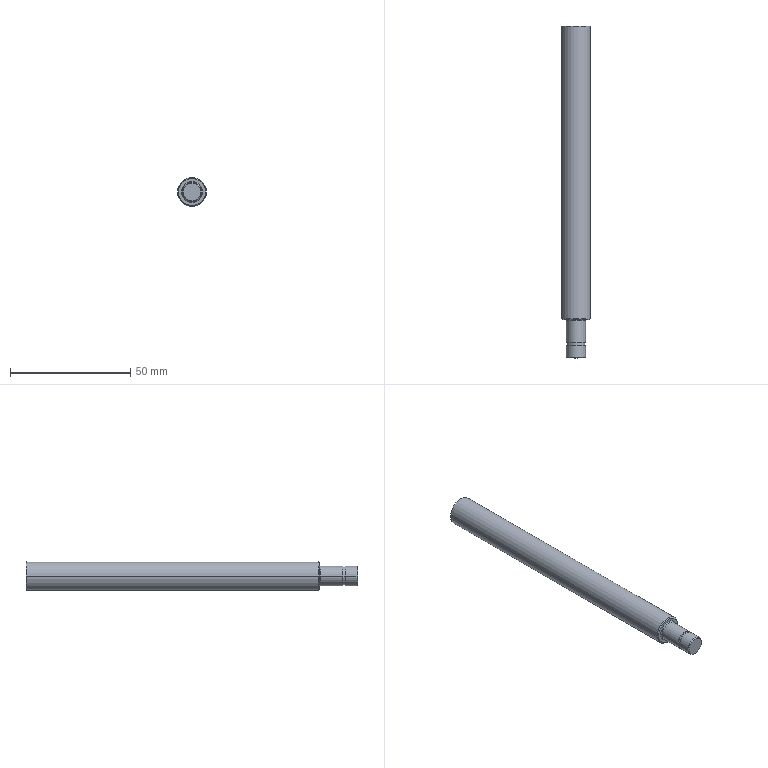Part | NX | features BREP 1 | 1 solid | 19 faces | box 12 x 138 x 12 mm | volume 14591 mm3 | cylinder 8 | plane 5 | cone 4 | torus 2 | commonest cylinder face diameters 8 x4 7.4 x2 12 x2
STEP:
#1=CARTESIAN_POINT('',(-6.,81.4,0.));
#2=VERTEX_POINT('',#1);
#3=CARTESIAN_POINT('',(-6.,203.,0.));
#4=VERTEX_POINT('',#3);
#5=CARTESIAN_POINT('',(-6.,65.,0.));
#6=DIRECTION('',(0.,1.,0.));
#7=VECTOR('',#6,1000.);
#8=LINE('',#5,#7);
#9=EDGE_CURVE('',#2,#4,#8,.T.);
#10=ORIENTED_EDGE('',*,*,#9,.T.);
#11=CARTESIAN_POINT('',(6.,203.,0.));
#12=VERTEX_POINT('',#11);
#13=CARTESIAN_POINT('',(0.,203.,0.));
#14=DIRECTION('',(0.,-1.,0.));
#15=DIRECTION('',(1.,0.,0.));
#16=AXIS2_PLACEMENT_3D('',#13,#14,#15);
#17=CIRCLE('',#16,6.);
#18=EDGE_CURVE('',#4,#12,#17,.T.);
#19=ORIENTED_EDGE('',*,*,#18,.T.);
#20=CARTESIAN_POINT('',(6.,81.4,0.));
#21=VERTEX_POINT('',#20);
#22=CARTESIAN_POINT('',(6.,65.,0.));
#23=DIRECTION('',(0.,-1.,0.));
#24=VECTOR('',#23,1000.);
#25=LINE('',#22,#24);
#26=EDGE_CURVE('',#12,#21,#25,.T.);
#27=ORIENTED_EDGE('',*,*,#26,.T.);
#28=CARTESIAN_POINT('',(0.,81.4,0.));
#29=DIRECTION('',(0.,1.,0.));
#30=DIRECTION('',(-1.,0.,0.));
#31=AXIS2_PLACEMENT_3D('',#28,#29,#30);
#32=CIRCLE('',#31,6.);
#33=EDGE_CURVE('',#21,#2,#32,.T.);
#34=ORIENTED_EDGE('',*,*,#33,.T.);
#35=EDGE_LOOP('',(#10,#19,#27,#34));
#36=FACE_BOUND('',#35,.T.);
#37=CARTESIAN_POINT('',(0.,65.,0.));
#38=DIRECTION('',(0.,-1.,0.));
#39=DIRECTION('',(1.,0.,0.));
#40=AXIS2_PLACEMENT_3D('',#37,#38,#39);
#41=CYLINDRICAL_SURFACE('',#40,6.);
#42=ADVANCED_FACE('',(#36),#41,.T.);
#43=ORIENTED_EDGE('',*,*,#26,.F.);
#44=CARTESIAN_POINT('',(0.,203.,0.));
#45=DIRECTION('',(0.,-1.,0.));
#46=DIRECTION('',(1.,0.,0.));
#47=AXIS2_PLACEMENT_3D('',#44,#45,#46);
#48=CIRCLE('',#47,6.);
#49=EDGE_CURVE('',#12,#4,#48,.T.);
#50=ORIENTED_EDGE('',*,*,#49,.T.);
#51=ORIENTED_EDGE('',*,*,#9,.F.);
#52=CARTESIAN_POINT('',(0.,81.4,0.));
#53=DIRECTION('',(0.,1.,0.));
#54=DIRECTION('',(-1.,0.,0.));
#55=AXIS2_PLACEMENT_3D('',#52,#53,#54);
#56=CIRCLE('',#55,6.);
#57=EDGE_CURVE('',#2,#21,#56,.T.);
#58=ORIENTED_EDGE('',*,*,#57,.T.);
#59=EDGE_LOOP('',(#43,#50,#51,#58));
#60=FACE_BOUND('',#59,.T.);
#61=CARTESIAN_POINT('',(0.,65.,0.));
#62=DIRECTION('',(0.,-1.,0.));
#63=DIRECTION('',(1.,0.,0.));
#64=AXIS2_PLACEMENT_3D('',#61,#62,#63);
#65=CYLINDRICAL_SURFACE('',#64,6.);
#66=ADVANCED_FACE('',(#60),#65,.T.);
#67=CARTESIAN_POINT('',(4.,80.6,0.));
#68=VERTEX_POINT('',#67);
#69=CARTESIAN_POINT('',(-4.,80.6,0.));
#70=VERTEX_POINT('',#69);
#71=CARTESIAN_POINT('',(0.,80.6,0.));
#72=DIRECTION('',(0.,-1.,0.));
#73=DIRECTION('',(-1.,0.,0.));
#74=AXIS2_PLACEMENT_3D('',#71,#72,#73);
#75=CIRCLE('',#74,4.);
#76=EDGE_CURVE('',#68,#70,#75,.T.);
#77=ORIENTED_EDGE('',*,*,#76,.F.);
#78=CARTESIAN_POINT('',(4.4,81.,0.));
#79=VERTEX_POINT('',#78);
#80=CARTESIAN_POINT('',(4.4,80.6,0.));
#81=DIRECTION('',(0.,0.,1.));
#82=DIRECTION('',(-1.,0.,0.));
#83=AXIS2_PLACEMENT_3D('',#80,#81,#82);
#84=CIRCLE('',#83,0.4);
#85=EDGE_CURVE('',#79,#68,#84,.T.);
#86=ORIENTED_EDGE('',*,*,#85,.F.);
#87=CARTESIAN_POINT('',(-4.4,81.,0.));
#88=VERTEX_POINT('',#87);
#89=CARTESIAN_POINT('',(0.,81.,0.));
#90=DIRECTION('',(0.,1.,0.));
#91=DIRECTION('',(-1.,0.,0.));
#92=AXIS2_PLACEMENT_3D('',#89,#90,#91);
#93=CIRCLE('',#92,4.4);
#94=EDGE_CURVE('',#88,#79,#93,.T.);
#95=ORIENTED_EDGE('',*,*,#94,.F.);
#96=CARTESIAN_POINT('',(-4.4,80.6,0.));
#97=DIRECTION('',(0.,0.,1.));
#98=DIRECTION('',(1.,0.,0.));
#99=AXIS2_PLACEMENT_3D('',#96,#97,#98);
#100=CIRCLE('',#99,0.4);
#101=EDGE_CURVE('',#70,#88,#100,.T.);
#102=ORIENTED_EDGE('',*,*,#101,.F.);
#103=EDGE_LOOP('',(#77,#86,#95,#102));
#104=FACE_BOUND('',#103,.T.);
#105=CARTESIAN_POINT('',(0.,80.6,0.));
#106=DIRECTION('',(0.,-1.,0.));
#107=DIRECTION('',(1.,0.,0.));
#108=AXIS2_PLACEMENT_3D('',#105,#106,#107);
#109=TOROIDAL_SURFACE('',#108,4.4,0.4);
#110=ADVANCED_FACE('',(#104),#109,.F.);
#111=CARTESIAN_POINT('',(-5.6,81.,0.));
#112=VERTEX_POINT('',#111);
#113=CARTESIAN_POINT('',(5.6,81.,0.));
#114=VERTEX_POINT('',#113);
#115=CARTESIAN_POINT('',(0.,81.,0.));
#116=DIRECTION('',(0.,-1.,0.));
#117=DIRECTION('',(-1.,0.,0.));
#118=AXIS2_PLACEMENT_3D('',#115,#116,#117);
#119=CIRCLE('',#118,5.6);
#120=EDGE_CURVE('',#112,#114,#119,.T.);
#121=ORIENTED_EDGE('',*,*,#120,.F.);
#122=CARTESIAN_POINT('',(-5.6,81.,0.));
#123=DIRECTION('',(-0.7071,0.7071,0.));
#124=VECTOR('',#123,1000.);
#125=LINE('',#122,#124);
#126=EDGE_CURVE('',#112,#2,#125,.T.);
#127=ORIENTED_EDGE('',*,*,#126,.T.);
#128=ORIENTED_EDGE('',*,*,#33,.F.);
#129=CARTESIAN_POINT('',(5.6,81.,0.));
#130=DIRECTION('',(-0.7071,-0.7071,0.));
#131=VECTOR('',#130,1000.);
#132=LINE('',#129,#131);
#133=EDGE_CURVE('',#21,#114,#132,.T.);
#134=ORIENTED_EDGE('',*,*,#133,.T.);
#135=EDGE_LOOP('',(#121,#127,#128,#134));
#136=FACE_BOUND('',#135,.T.);
#137=CARTESIAN_POINT('',(0.,81.,0.));
#138=DIRECTION('',(0.,1.,0.));
#139=DIRECTION('',(-1.,0.,0.));
#140=AXIS2_PLACEMENT_3D('',#137,#138,#139);
#141=CONICAL_SURFACE('',#140,5.6,0.7854);
#142=ADVANCED_FACE('',(#136),#141,.T.);
#143=CARTESIAN_POINT('',(-3.6,65.,0.));
#144=VERTEX_POINT('',#143);
#145=CARTESIAN_POINT('',(3.6,65.,0.));
#146=VERTEX_POINT('',#145);
#147=CARTESIAN_POINT('',(0.,65.,0.));
#148=DIRECTION('',(0.,-1.,0.));
#149=DIRECTION('',(-1.,0.,0.));
#150=AXIS2_PLACEMENT_3D('',#147,#148,#149);
#151=CIRCLE('',#150,3.6);
#152=EDGE_CURVE('',#144,#146,#151,.T.);
#153=ORIENTED_EDGE('',*,*,#152,.F.);
#154=CARTESIAN_POINT('',(-4.,65.4,0.));
#155=VERTEX_POINT('',#154);
#156=CARTESIAN_POINT('',(-3.6,65.,0.));
#157=DIRECTION('',(-0.7071,0.7071,0.));
#158=VECTOR('',#157,1000.);
#159=LINE('',#156,#158);
#160=EDGE_CURVE('',#144,#155,#159,.T.);
#161=ORIENTED_EDGE('',*,*,#160,.T.);
#162=CARTESIAN_POINT('',(4.,65.4,0.));
#163=VERTEX_POINT('',#162);
#164=CARTESIAN_POINT('',(0.,65.4,0.));
#165=DIRECTION('',(0.,1.,0.));
#166=DIRECTION('',(-1.,0.,0.));
#167=AXIS2_PLACEMENT_3D('',#164,#165,#166);
#168=CIRCLE('',#167,4.);
#169=EDGE_CURVE('',#163,#155,#168,.T.);
#170=ORIENTED_EDGE('',*,*,#169,.F.);
#171=CARTESIAN_POINT('',(3.6,65.,0.));
#172=DIRECTION('',(-0.7071,-0.7071,0.));
#173=VECTOR('',#172,1000.);
#174=LINE('',#171,#173);
#175=EDGE_CURVE('',#163,#146,#174,.T.);
#176=ORIENTED_EDGE('',*,*,#175,.T.);
#177=EDGE_LOOP('',(#153,#161,#170,#176));
#178=FACE_BOUND('',#177,.T.);
#179=CARTESIAN_POINT('',(0.,65.,0.));
#180=DIRECTION('',(0.,1.,0.));
#181=DIRECTION('',(-1.,0.,0.));
#182=AXIS2_PLACEMENT_3D('',#179,#180,#181);
#183=CONICAL_SURFACE('',#182,3.6,0.7854);
#184=ADVANCED_FACE('',(#178),#183,.T.);
#185=CARTESIAN_POINT('',(-4.,70.3,0.));
#186=VERTEX_POINT('',#185);
#187=CARTESIAN_POINT('',(4.,70.3,0.));
#188=VERTEX_POINT('',#187);
#189=CARTESIAN_POINT('',(0.,70.3,0.));
#190=DIRECTION('',(0.,-1.,0.));
#191=DIRECTION('',(-1.,0.,0.));
#192=AXIS2_PLACEMENT_3D('',#189,#190,#191);
#193=CIRCLE('',#192,4.);
#194=EDGE_CURVE('',#186,#188,#193,.T.);
#195=ORIENTED_EDGE('',*,*,#194,.T.);
#196=CARTESIAN_POINT('',(4.,65.,0.));
#197=DIRECTION('',(0.,1.,0.));
#198=VECTOR('',#197,1000.);
#199=LINE('',#196,#198);
#200=EDGE_CURVE('',#163,#188,#199,.T.);
#201=ORIENTED_EDGE('',*,*,#200,.F.);
#202=ORIENTED_EDGE('',*,*,#169,.T.);
#203=CARTESIAN_POINT('',(-4.,65.,0.));
#204=DIRECTION('',(0.,-1.,0.));
#205=VECTOR('',#204,1000.);
#206=LINE('',#203,#205);
#207=EDGE_CURVE('',#186,#155,#206,.T.);
#208=ORIENTED_EDGE('',*,*,#207,.F.);
#209=EDGE_LOOP('',(#195,#201,#202,#208));
#210=FACE_BOUND('',#209,.T.);
#211=CARTESIAN_POINT('',(0.,65.,0.));
#212=DIRECTION('',(0.,-1.,0.));
#213=DIRECTION('',(1.,0.,0.));
#214=AXIS2_PLACEMENT_3D('',#211,#212,#213);
#215=CYLINDRICAL_SURFACE('',#214,4.);
#216=ADVANCED_FACE('',(#210),#215,.T.);
#217=CARTESIAN_POINT('',(-3.7,71.3,0.));
#218=VERTEX_POINT('',#217);
#219=CARTESIAN_POINT('',(3.7,71.3,0.));
#220=VERTEX_POINT('',#219);
#221=CARTESIAN_POINT('',(0.,71.3,0.));
#222=DIRECTION('',(0.,-1.,0.));
#223=DIRECTION('',(-1.,0.,0.));
#224=AXIS2_PLACEMENT_3D('',#221,#222,#223);
#225=CIRCLE('',#224,3.7);
#226=EDGE_CURVE('',#218,#220,#225,.T.);
#227=ORIENTED_EDGE('',*,*,#226,.T.);
#228=CARTESIAN_POINT('',(3.7,70.3,0.));
#229=VERTEX_POINT('',#228);
#230=CARTESIAN_POINT('',(3.7,65.,0.));
#231=DIRECTION('',(0.,1.,0.));
#232=VECTOR('',#231,1000.);
#233=LINE('',#230,#232);
#234=EDGE_CURVE('',#229,#220,#233,.T.);
#235=ORIENTED_EDGE('',*,*,#234,.F.);
#236=CARTESIAN_POINT('',(-3.7,70.3,0.));
#237=VERTEX_POINT('',#236);
#238=CARTESIAN_POINT('',(0.,70.3,0.));
#239=DIRECTION('',(0.,-1.,0.));
#240=DIRECTION('',(-1.,0.,0.));
#241=AXIS2_PLACEMENT_3D('',#238,#239,#240);
#242=CIRCLE('',#241,3.7);
#243=EDGE_CURVE('',#237,#229,#242,.T.);
#244=ORIENTED_EDGE('',*,*,#243,.F.);
#245=CARTESIAN_POINT('',(-3.7,65.,0.));
#246=DIRECTION('',(0.,-1.,0.));
#247=VECTOR('',#246,1000.);
#248=LINE('',#245,#247);
#249=EDGE_CURVE('',#218,#237,#248,.T.);
#250=ORIENTED_EDGE('',*,*,#249,.F.);
#251=EDGE_LOOP('',(#227,#235,#244,#250));
#252=FACE_BOUND('',#251,.T.);
#253=CARTESIAN_POINT('',(0.,65.,0.));
#254=DIRECTION('',(0.,-1.,0.));
#255=DIRECTION('',(1.,0.,0.));
#256=AXIS2_PLACEMENT_3D('',#253,#254,#255);
#257=CYLINDRICAL_SURFACE('',#256,3.7);
#258=ADVANCED_FACE('',(#252),#257,.T.);
#259=CARTESIAN_POINT('',(0.,80.6,0.));
#260=DIRECTION('',(0.,-1.,0.));
#261=DIRECTION('',(-1.,0.,0.));
#262=AXIS2_PLACEMENT_3D('',#259,#260,#261);
#263=CIRCLE('',#262,4.);
#264=EDGE_CURVE('',#70,#68,#263,.T.);
#265=ORIENTED_EDGE('',*,*,#264,.T.);
#266=CARTESIAN_POINT('',(4.,71.3,0.));
#267=VERTEX_POINT('',#266);
#268=CARTESIAN_POINT('',(4.,65.,0.));
#269=DIRECTION('',(0.,1.,0.));
#270=VECTOR('',#269,1000.);
#271=LINE('',#268,#270);
#272=EDGE_CURVE('',#267,#68,#271,.T.);
#273=ORIENTED_EDGE('',*,*,#272,.F.);
#274=CARTESIAN_POINT('',(-4.,71.3,0.));
#275=VERTEX_POINT('',#274);
#276=CARTESIAN_POINT('',(0.,71.3,0.));
#277=DIRECTION('',(0.,-1.,0.));
#278=DIRECTION('',(-1.,0.,0.));
#279=AXIS2_PLACEMENT_3D('',#276,#277,#278);
#280=CIRCLE('',#279,4.);
#281=EDGE_CURVE('',#275,#267,#280,.T.);
#282=ORIENTED_EDGE('',*,*,#281,.F.);
#283=CARTESIAN_POINT('',(-4.,65.,0.));
#284=DIRECTION('',(0.,-1.,0.));
#285=VECTOR('',#284,1000.);
#286=LINE('',#283,#285);
#287=EDGE_CURVE('',#70,#275,#286,.T.);
#288=ORIENTED_EDGE('',*,*,#287,.F.);
#289=EDGE_LOOP('',(#265,#273,#282,#288));
#290=FACE_BOUND('',#289,.T.);
#291=CARTESIAN_POINT('',(0.,65.,0.));
#292=DIRECTION('',(0.,-1.,0.));
#293=DIRECTION('',(1.,0.,0.));
#294=AXIS2_PLACEMENT_3D('',#291,#292,#293);
#295=CYLINDRICAL_SURFACE('',#294,4.);
#296=ADVANCED_FACE('',(#290),#295,.T.);
#297=ORIENTED_EDGE('',*,*,#272,.T.);
#298=ORIENTED_EDGE('',*,*,#76,.T.);
#299=ORIENTED_EDGE('',*,*,#287,.T.);
#300=CARTESIAN_POINT('',(0.,71.3,0.));
#301=DIRECTION('',(0.,-1.,0.));
#302=DIRECTION('',(-1.,0.,0.));
#303=AXIS2_PLACEMENT_3D('',#300,#301,#302);
#304=CIRCLE('',#303,4.);
#305=EDGE_CURVE('',#267,#275,#304,.T.);
#306=ORIENTED_EDGE('',*,*,#305,.F.);
#307=EDGE_LOOP('',(#297,#298,#299,#306));
#308=FACE_BOUND('',#307,.T.);
#309=CARTESIAN_POINT('',(0.,65.,0.));
#310=DIRECTION('',(0.,-1.,0.));
#311=DIRECTION('',(1.,0.,0.));
#312=AXIS2_PLACEMENT_3D('',#309,#310,#311);
#313=CYLINDRICAL_SURFACE('',#312,4.);
#314=ADVANCED_FACE('',(#308),#313,.T.);
#315=ORIENTED_EDGE('',*,*,#226,.F.);
#316=CARTESIAN_POINT('',(0.,71.3,0.));
#317=DIRECTION('',(0.,-1.,0.));
#318=DIRECTION('',(-1.,0.,0.));
#319=AXIS2_PLACEMENT_3D('',#316,#317,#318);
#320=CIRCLE('',#319,3.7);
#321=EDGE_CURVE('',#220,#218,#320,.T.);
#322=ORIENTED_EDGE('',*,*,#321,.F.);
#323=EDGE_LOOP('',(#315,#322));
#324=FACE_BOUND('',#323,.T.);
#325=ORIENTED_EDGE('',*,*,#281,.T.);
#326=ORIENTED_EDGE('',*,*,#305,.T.);
#327=EDGE_LOOP('',(#325,#326));
#328=FACE_BOUND('',#327,.T.);
#329=CARTESIAN_POINT('',(0.,71.3,0.));
#330=DIRECTION('',(0.,1.,0.));
#331=DIRECTION('',(-1.,0.,0.));
#332=AXIS2_PLACEMENT_3D('',#329,#330,#331);
#333=PLANE('',#332);
#334=ADVANCED_FACE('',(#324,#328),#333,.F.);
#335=ORIENTED_EDGE('',*,*,#234,.T.);
#336=ORIENTED_EDGE('',*,*,#321,.T.);
#337=ORIENTED_EDGE('',*,*,#249,.T.);
#338=CARTESIAN_POINT('',(0.,70.3,0.));
#339=DIRECTION('',(0.,-1.,0.));
#340=DIRECTION('',(-1.,0.,0.));
#341=AXIS2_PLACEMENT_3D('',#338,#339,#340);
#342=CIRCLE('',#341,3.7);
#343=EDGE_CURVE('',#229,#237,#342,.T.);
#344=ORIENTED_EDGE('',*,*,#343,.F.);
#345=EDGE_LOOP('',(#335,#336,#337,#344));
#346=FACE_BOUND('',#345,.T.);
#347=CARTESIAN_POINT('',(0.,65.,0.));
#348=DIRECTION('',(0.,-1.,0.));
#349=DIRECTION('',(1.,0.,0.));
#350=AXIS2_PLACEMENT_3D('',#347,#348,#349);
#351=CYLINDRICAL_SURFACE('',#350,3.7);
#352=ADVANCED_FACE('',(#346),#351,.T.);
#353=ORIENTED_EDGE('',*,*,#243,.T.);
#354=ORIENTED_EDGE('',*,*,#343,.T.);
#355=EDGE_LOOP('',(#353,#354));
#356=FACE_BOUND('',#355,.T.);
#357=ORIENTED_EDGE('',*,*,#194,.F.);
#358=CARTESIAN_POINT('',(0.,70.3,0.));
#359=DIRECTION('',(0.,-1.,0.));
#360=DIRECTION('',(-1.,0.,0.));
#361=AXIS2_PLACEMENT_3D('',#358,#359,#360);
#362=CIRCLE('',#361,4.);
#363=EDGE_CURVE('',#188,#186,#362,.T.);
#364=ORIENTED_EDGE('',*,*,#363,.F.);
#365=EDGE_LOOP('',(#357,#364));
#366=FACE_BOUND('',#365,.T.);
#367=CARTESIAN_POINT('',(0.,70.3,0.));
#368=DIRECTION('',(0.,1.,0.));
#369=DIRECTION('',(-1.,0.,0.));
#370=AXIS2_PLACEMENT_3D('',#367,#368,#369);
#371=PLANE('',#370);
#372=ADVANCED_FACE('',(#356,#366),#371,.T.);
#373=ORIENTED_EDGE('',*,*,#200,.T.);
#374=ORIENTED_EDGE('',*,*,#363,.T.);
#375=ORIENTED_EDGE('',*,*,#207,.T.);
#376=CARTESIAN_POINT('',(0.,65.4,0.));
#377=DIRECTION('',(0.,1.,0.));
#378=DIRECTION('',(-1.,0.,0.));
#379=AXIS2_PLACEMENT_3D('',#376,#377,#378);
#380=CIRCLE('',#379,4.);
#381=EDGE_CURVE('',#155,#163,#380,.T.);
#382=ORIENTED_EDGE('',*,*,#381,.T.);
#383=EDGE_LOOP('',(#373,#374,#375,#382));
#384=FACE_BOUND('',#383,.T.);
#385=CARTESIAN_POINT('',(0.,65.,0.));
#386=DIRECTION('',(0.,-1.,0.));
#387=DIRECTION('',(1.,0.,0.));
#388=AXIS2_PLACEMENT_3D('',#385,#386,#387);
#389=CYLINDRICAL_SURFACE('',#388,4.);
#390=ADVANCED_FACE('',(#384),#389,.T.);
#391=CARTESIAN_POINT('',(0.,65.,0.));
#392=DIRECTION('',(0.,-1.,0.));
#393=DIRECTION('',(-1.,0.,0.));
#394=AXIS2_PLACEMENT_3D('',#391,#392,#393);
#395=CIRCLE('',#394,3.6);
#396=EDGE_CURVE('',#146,#144,#395,.T.);
#397=ORIENTED_EDGE('',*,*,#396,.T.);
#398=ORIENTED_EDGE('',*,*,#152,.T.);
#399=EDGE_LOOP('',(#397,#398));
#400=FACE_BOUND('',#399,.T.);
#401=CARTESIAN_POINT('',(0.,65.,0.));
#402=DIRECTION('',(0.,-1.,0.));
#403=DIRECTION('',(1.,0.,0.));
#404=AXIS2_PLACEMENT_3D('',#401,#402,#403);
#405=PLANE('',#404);
#406=ADVANCED_FACE('',(#400),#405,.T.);
#407=ORIENTED_EDGE('',*,*,#94,.T.);
#408=CARTESIAN_POINT('',(0.,81.,0.));
#409=DIRECTION('',(0.,1.,0.));
#410=DIRECTION('',(-1.,0.,0.));
#411=AXIS2_PLACEMENT_3D('',#408,#409,#410);
#412=CIRCLE('',#411,4.4);
#413=EDGE_CURVE('',#79,#88,#412,.T.);
#414=ORIENTED_EDGE('',*,*,#413,.T.);
#415=EDGE_LOOP('',(#407,#414));
#416=FACE_BOUND('',#415,.T.);
#417=CARTESIAN_POINT('',(0.,81.,0.));
#418=DIRECTION('',(0.,-1.,0.));
#419=DIRECTION('',(-1.,0.,0.));
#420=AXIS2_PLACEMENT_3D('',#417,#418,#419);
#421=CIRCLE('',#420,5.6);
#422=EDGE_CURVE('',#114,#112,#421,.T.);
#423=ORIENTED_EDGE('',*,*,#422,.T.);
#424=ORIENTED_EDGE('',*,*,#120,.T.);
#425=EDGE_LOOP('',(#423,#424));
#426=FACE_BOUND('',#425,.T.);
#427=CARTESIAN_POINT('',(0.,81.,0.));
#428=DIRECTION('',(0.,-1.,0.));
#429=DIRECTION('',(1.,0.,0.));
#430=AXIS2_PLACEMENT_3D('',#427,#428,#429);
#431=PLANE('',#430);
#432=ADVANCED_FACE('',(#416,#426),#431,.T.);
#433=ORIENTED_EDGE('',*,*,#160,.F.);
#434=ORIENTED_EDGE('',*,*,#396,.F.);
#435=ORIENTED_EDGE('',*,*,#175,.F.);
#436=ORIENTED_EDGE('',*,*,#381,.F.);
#437=EDGE_LOOP('',(#433,#434,#435,#436));
#438=FACE_BOUND('',#437,.T.);
#439=CARTESIAN_POINT('',(0.,65.,0.));
#440=DIRECTION('',(0.,1.,0.));
#441=DIRECTION('',(-1.,0.,0.));
#442=AXIS2_PLACEMENT_3D('',#439,#440,#441);
#443=CONICAL_SURFACE('',#442,3.6,0.7854);
#444=ADVANCED_FACE('',(#438),#443,.T.);
#445=ORIENTED_EDGE('',*,*,#126,.F.);
#446=ORIENTED_EDGE('',*,*,#422,.F.);
#447=ORIENTED_EDGE('',*,*,#133,.F.);
#448=ORIENTED_EDGE('',*,*,#57,.F.);
#449=EDGE_LOOP('',(#445,#446,#447,#448));
#450=FACE_BOUND('',#449,.T.);
#451=CARTESIAN_POINT('',(0.,81.,0.));
#452=DIRECTION('',(0.,1.,0.));
#453=DIRECTION('',(-1.,0.,0.));
#454=AXIS2_PLACEMENT_3D('',#451,#452,#453);
#455=CONICAL_SURFACE('',#454,5.6,0.7854);
#456=ADVANCED_FACE('',(#450),#455,.T.);
#457=ORIENTED_EDGE('',*,*,#85,.T.);
#458=ORIENTED_EDGE('',*,*,#264,.F.);
#459=ORIENTED_EDGE('',*,*,#101,.T.);
#460=ORIENTED_EDGE('',*,*,#413,.F.);
#461=EDGE_LOOP('',(#457,#458,#459,#460));
#462=FACE_BOUND('',#461,.T.);
#463=CARTESIAN_POINT('',(0.,80.6,0.));
#464=DIRECTION('',(0.,-1.,0.));
#465=DIRECTION('',(1.,0.,0.));
#466=AXIS2_PLACEMENT_3D('',#463,#464,#465);
#467=TOROIDAL_SURFACE('',#466,4.4,0.4);
#468=ADVANCED_FACE('',(#462),#467,.F.);
#469=ORIENTED_EDGE('',*,*,#49,.F.);
#470=ORIENTED_EDGE('',*,*,#18,.F.);
#471=EDGE_LOOP('',(#469,#470));
#472=FACE_BOUND('',#471,.T.);
#473=CARTESIAN_POINT('',(0.,203.,0.));
#474=DIRECTION('',(0.,1.,0.));
#475=DIRECTION('',(1.,0.,0.));
#476=AXIS2_PLACEMENT_3D('',#473,#474,#475);
#477=PLANE('',#476);
#478=ADVANCED_FACE('',(#472),#477,.T.);
#479=CLOSED_SHELL('',(#42,#66,#110,#142,#184,#216,#258,#296,#314,#334,#352,#372,#390,#406,#432,#444,#456,#468,#478));
#480=MANIFOLD_SOLID_BREP('',#479);
#481=(LENGTH_UNIT()NAMED_UNIT(*)SI_UNIT(.MILLI.,.METRE.));
#482=UNCERTAINTY_MEASURE_WITH_UNIT(LENGTH_MEASURE(0.00001),#481,'','');
#483=(NAMED_UNIT(*)PLANE_ANGLE_UNIT()SI_UNIT($,.RADIAN.));
#484=(NAMED_UNIT(*)SI_UNIT($,.STERADIAN.)SOLID_ANGLE_UNIT());
#485=(GEOMETRIC_REPRESENTATION_CONTEXT(3)GLOBAL_UNCERTAINTY_ASSIGNED_CONTEXT((#482))GLOBAL_UNIT_ASSIGNED_CONTEXT((#481,#483,#484))REPRESENTATION_CONTEXT('',''));
#486=ADVANCED_BREP_SHAPE_REPRESENTATION('',(#480),#485);